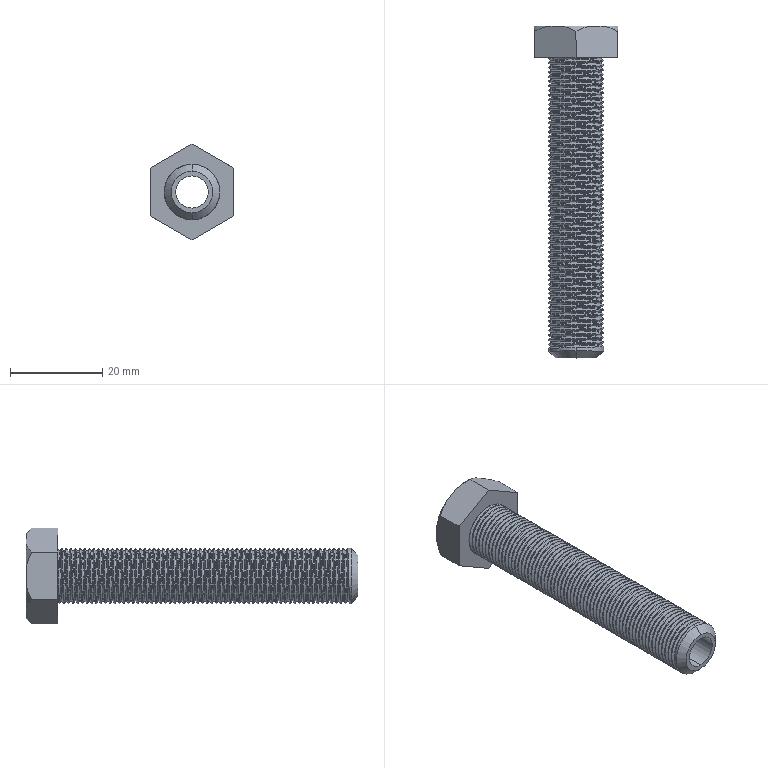Part | SolidWorks | features ICE 2, Chamfer 1, Extrusion 1, RevCut 1, SweepThread 1 | 1 solid | 159 faces | box 18 x 71.9 x 20.785 mm | volume 5747 mm3 | cylinder 136 | plane 11 | cone 9 | spline 3 | commonest cylinder face diameters 12 x134 7 x2